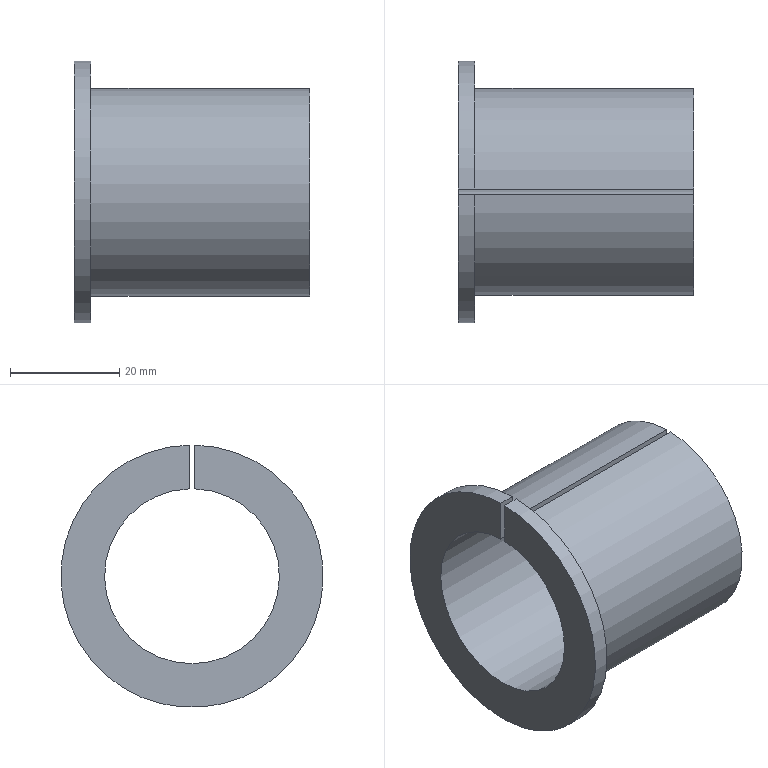Part | STEP file | HXGR200008-05-22-05 | 1 solid | 8 faces | box 43 x 48 x 47.995 mm | volume 16067 mm3 | plane 5 | cylinder 3 | commonest cylinder face diameters 32 x1 38 x1 48 x1
STEP:
#1=CARTESIAN_POINT('',(0.,0.5,23.995));
#2=VERTEX_POINT('',#1);
#3=CARTESIAN_POINT('',(0.,-0.5,23.995));
#4=VERTEX_POINT('',#3);
#5=CARTESIAN_POINT('',(0.,0.,0.));
#6=DIRECTION('',(-1.,0.,0.));
#7=DIRECTION('',(0.,0.,1.));
#8=AXIS2_PLACEMENT_3D('',#5,#6,#7);
#9=CIRCLE('',#8,24.);
#10=EDGE_CURVE('',#2,#4,#9,.T.);
#11=ORIENTED_EDGE('',*,*,#10,.F.);
#12=CARTESIAN_POINT('',(3.,0.5,23.995));
#13=VERTEX_POINT('',#12);
#14=CARTESIAN_POINT('',(0.,0.5,23.995));
#15=DIRECTION('',(-1.,0.,0.));
#16=VECTOR('',#15,1000.);
#17=LINE('',#14,#16);
#18=EDGE_CURVE('',#13,#2,#17,.T.);
#19=ORIENTED_EDGE('',*,*,#18,.F.);
#20=CARTESIAN_POINT('',(3.,-0.5,23.995));
#21=VERTEX_POINT('',#20);
#22=CARTESIAN_POINT('',(3.,0.,0.));
#23=DIRECTION('',(-1.,0.,0.));
#24=DIRECTION('',(0.,0.,1.));
#25=AXIS2_PLACEMENT_3D('',#22,#23,#24);
#26=CIRCLE('',#25,24.);
#27=EDGE_CURVE('',#13,#21,#26,.T.);
#28=ORIENTED_EDGE('',*,*,#27,.T.);
#29=CARTESIAN_POINT('',(0.,-0.5,23.995));
#30=DIRECTION('',(1.,0.,0.));
#31=VECTOR('',#30,1000.);
#32=LINE('',#29,#31);
#33=EDGE_CURVE('',#4,#21,#32,.T.);
#34=ORIENTED_EDGE('',*,*,#33,.F.);
#35=EDGE_LOOP('',(#11,#19,#28,#34));
#36=FACE_OUTER_BOUND('',#35,.T.);
#37=CARTESIAN_POINT('',(0.,0.,0.));
#38=DIRECTION('',(-1.,0.,0.));
#39=DIRECTION('',(0.,0.,1.));
#40=AXIS2_PLACEMENT_3D('',#37,#38,#39);
#41=CYLINDRICAL_SURFACE('',#40,24.);
#42=ADVANCED_FACE('',(#36),#41,.T.);
#43=CARTESIAN_POINT('',(0.,0.5,15.992));
#44=VERTEX_POINT('',#43);
#45=CARTESIAN_POINT('',(0.,-0.5,15.992));
#46=VERTEX_POINT('',#45);
#47=CARTESIAN_POINT('',(0.,0.,0.));
#48=DIRECTION('',(-1.,0.,0.));
#49=DIRECTION('',(0.,0.,1.));
#50=AXIS2_PLACEMENT_3D('',#47,#48,#49);
#51=CIRCLE('',#50,16.);
#52=EDGE_CURVE('',#44,#46,#51,.T.);
#53=ORIENTED_EDGE('',*,*,#52,.F.);
#54=CARTESIAN_POINT('',(0.,0.5,48.));
#55=DIRECTION('',(0.,0.,-1.));
#56=VECTOR('',#55,1000.);
#57=LINE('',#54,#56);
#58=EDGE_CURVE('',#2,#44,#57,.T.);
#59=ORIENTED_EDGE('',*,*,#58,.F.);
#60=ORIENTED_EDGE('',*,*,#10,.T.);
#61=CARTESIAN_POINT('',(0.,-0.5,48.));
#62=DIRECTION('',(0.,0.,1.));
#63=VECTOR('',#62,1000.);
#64=LINE('',#61,#63);
#65=EDGE_CURVE('',#46,#4,#64,.T.);
#66=ORIENTED_EDGE('',*,*,#65,.F.);
#67=EDGE_LOOP('',(#53,#59,#60,#66));
#68=FACE_OUTER_BOUND('',#67,.T.);
#69=CARTESIAN_POINT('',(0.,24.,0.));
#70=DIRECTION('',(1.,0.,0.));
#71=DIRECTION('',(0.,0.,-1.));
#72=AXIS2_PLACEMENT_3D('',#69,#70,#71);
#73=PLANE('',#72);
#74=ADVANCED_FACE('',(#68),#73,.F.);
#75=CARTESIAN_POINT('',(43.,0.5,15.992));
#76=VERTEX_POINT('',#75);
#77=CARTESIAN_POINT('',(43.,-0.5,15.992));
#78=VERTEX_POINT('',#77);
#79=CARTESIAN_POINT('',(43.,0.,0.));
#80=DIRECTION('',(-1.,0.,0.));
#81=DIRECTION('',(0.,0.,1.));
#82=AXIS2_PLACEMENT_3D('',#79,#80,#81);
#83=CIRCLE('',#82,16.);
#84=EDGE_CURVE('',#76,#78,#83,.T.);
#85=ORIENTED_EDGE('',*,*,#84,.F.);
#86=CARTESIAN_POINT('',(0.,0.5,15.992));
#87=DIRECTION('',(1.,0.,0.));
#88=VECTOR('',#87,1000.);
#89=LINE('',#86,#88);
#90=EDGE_CURVE('',#44,#76,#89,.T.);
#91=ORIENTED_EDGE('',*,*,#90,.F.);
#92=ORIENTED_EDGE('',*,*,#52,.T.);
#93=CARTESIAN_POINT('',(0.,-0.5,15.992));
#94=DIRECTION('',(-1.,0.,0.));
#95=VECTOR('',#94,1000.);
#96=LINE('',#93,#95);
#97=EDGE_CURVE('',#78,#46,#96,.T.);
#98=ORIENTED_EDGE('',*,*,#97,.F.);
#99=EDGE_LOOP('',(#85,#91,#92,#98));
#100=FACE_OUTER_BOUND('',#99,.T.);
#101=CARTESIAN_POINT('',(0.,0.,0.));
#102=DIRECTION('',(-1.,0.,0.));
#103=DIRECTION('',(0.,0.,1.));
#104=AXIS2_PLACEMENT_3D('',#101,#102,#103);
#105=CYLINDRICAL_SURFACE('',#104,16.);
#106=ADVANCED_FACE('',(#100),#105,.F.);
#107=CARTESIAN_POINT('',(43.,0.5,18.993));
#108=VERTEX_POINT('',#107);
#109=CARTESIAN_POINT('',(43.,-0.5,18.993));
#110=VERTEX_POINT('',#109);
#111=CARTESIAN_POINT('',(43.,0.,0.));
#112=DIRECTION('',(-1.,0.,0.));
#113=DIRECTION('',(0.,0.,1.));
#114=AXIS2_PLACEMENT_3D('',#111,#112,#113);
#115=CIRCLE('',#114,19.);
#116=EDGE_CURVE('',#108,#110,#115,.T.);
#117=ORIENTED_EDGE('',*,*,#116,.F.);
#118=CARTESIAN_POINT('',(43.,0.5,48.));
#119=DIRECTION('',(0.,0.,1.));
#120=VECTOR('',#119,1000.);
#121=LINE('',#118,#120);
#122=EDGE_CURVE('',#76,#108,#121,.T.);
#123=ORIENTED_EDGE('',*,*,#122,.F.);
#124=ORIENTED_EDGE('',*,*,#84,.T.);
#125=CARTESIAN_POINT('',(43.,-0.5,48.));
#126=DIRECTION('',(0.,0.,-1.));
#127=VECTOR('',#126,1000.);
#128=LINE('',#125,#127);
#129=EDGE_CURVE('',#110,#78,#128,.T.);
#130=ORIENTED_EDGE('',*,*,#129,.F.);
#131=EDGE_LOOP('',(#117,#123,#124,#130));
#132=FACE_OUTER_BOUND('',#131,.T.);
#133=CARTESIAN_POINT('',(43.,16.,0.));
#134=DIRECTION('',(-1.,0.,0.));
#135=DIRECTION('',(0.,0.,1.));
#136=AXIS2_PLACEMENT_3D('',#133,#134,#135);
#137=PLANE('',#136);
#138=ADVANCED_FACE('',(#132),#137,.F.);
#139=CARTESIAN_POINT('',(3.,0.5,18.993));
#140=VERTEX_POINT('',#139);
#141=CARTESIAN_POINT('',(3.,-0.5,18.993));
#142=VERTEX_POINT('',#141);
#143=CARTESIAN_POINT('',(3.,0.,0.));
#144=DIRECTION('',(-1.,0.,0.));
#145=DIRECTION('',(0.,0.,1.));
#146=AXIS2_PLACEMENT_3D('',#143,#144,#145);
#147=CIRCLE('',#146,19.);
#148=EDGE_CURVE('',#140,#142,#147,.T.);
#149=ORIENTED_EDGE('',*,*,#148,.F.);
#150=CARTESIAN_POINT('',(0.,0.5,18.993));
#151=DIRECTION('',(-1.,0.,0.));
#152=VECTOR('',#151,1000.);
#153=LINE('',#150,#152);
#154=EDGE_CURVE('',#108,#140,#153,.T.);
#155=ORIENTED_EDGE('',*,*,#154,.F.);
#156=ORIENTED_EDGE('',*,*,#116,.T.);
#157=CARTESIAN_POINT('',(0.,-0.5,18.993));
#158=DIRECTION('',(1.,0.,0.));
#159=VECTOR('',#158,1000.);
#160=LINE('',#157,#159);
#161=EDGE_CURVE('',#142,#110,#160,.T.);
#162=ORIENTED_EDGE('',*,*,#161,.F.);
#163=EDGE_LOOP('',(#149,#155,#156,#162));
#164=FACE_OUTER_BOUND('',#163,.T.);
#165=CARTESIAN_POINT('',(0.,0.,0.));
#166=DIRECTION('',(-1.,0.,0.));
#167=DIRECTION('',(0.,0.,1.));
#168=AXIS2_PLACEMENT_3D('',#165,#166,#167);
#169=CYLINDRICAL_SURFACE('',#168,19.);
#170=ADVANCED_FACE('',(#164),#169,.T.);
#171=ORIENTED_EDGE('',*,*,#27,.F.);
#172=CARTESIAN_POINT('',(3.,0.5,48.));
#173=DIRECTION('',(0.,0.,1.));
#174=VECTOR('',#173,1000.);
#175=LINE('',#172,#174);
#176=EDGE_CURVE('',#140,#13,#175,.T.);
#177=ORIENTED_EDGE('',*,*,#176,.F.);
#178=ORIENTED_EDGE('',*,*,#148,.T.);
#179=CARTESIAN_POINT('',(3.,-0.5,48.));
#180=DIRECTION('',(0.,0.,-1.));
#181=VECTOR('',#180,1000.);
#182=LINE('',#179,#181);
#183=EDGE_CURVE('',#21,#142,#182,.T.);
#184=ORIENTED_EDGE('',*,*,#183,.F.);
#185=EDGE_LOOP('',(#171,#177,#178,#184));
#186=FACE_OUTER_BOUND('',#185,.T.);
#187=CARTESIAN_POINT('',(3.,19.,0.));
#188=DIRECTION('',(-1.,0.,0.));
#189=DIRECTION('',(0.,0.,1.));
#190=AXIS2_PLACEMENT_3D('',#187,#188,#189);
#191=PLANE('',#190);
#192=ADVANCED_FACE('',(#186),#191,.F.);
#193=ORIENTED_EDGE('',*,*,#33,.T.);
#194=ORIENTED_EDGE('',*,*,#183,.T.);
#195=ORIENTED_EDGE('',*,*,#161,.T.);
#196=ORIENTED_EDGE('',*,*,#129,.T.);
#197=ORIENTED_EDGE('',*,*,#97,.T.);
#198=ORIENTED_EDGE('',*,*,#65,.T.);
#199=EDGE_LOOP('',(#193,#194,#195,#196,#197,#198));
#200=FACE_OUTER_BOUND('',#199,.T.);
#201=CARTESIAN_POINT('',(43.001,-0.5,48.));
#202=DIRECTION('',(0.,-1.,0.));
#203=DIRECTION('',(0.,0.,-1.));
#204=AXIS2_PLACEMENT_3D('',#201,#202,#203);
#205=PLANE('',#204);
#206=ADVANCED_FACE('',(#200),#205,.F.);
#207=ORIENTED_EDGE('',*,*,#18,.T.);
#208=ORIENTED_EDGE('',*,*,#58,.T.);
#209=ORIENTED_EDGE('',*,*,#90,.T.);
#210=ORIENTED_EDGE('',*,*,#122,.T.);
#211=ORIENTED_EDGE('',*,*,#154,.T.);
#212=ORIENTED_EDGE('',*,*,#176,.T.);
#213=EDGE_LOOP('',(#207,#208,#209,#210,#211,#212));
#214=FACE_OUTER_BOUND('',#213,.T.);
#215=CARTESIAN_POINT('',(43.001,0.5,48.));
#216=DIRECTION('',(0.,1.,0.));
#217=DIRECTION('',(0.,0.,1.));
#218=AXIS2_PLACEMENT_3D('',#215,#216,#217);
#219=PLANE('',#218);
#220=ADVANCED_FACE('',(#214),#219,.F.);
#221=CLOSED_SHELL('',(#42,#74,#106,#138,#170,#192,#206,#220));
#222=MANIFOLD_SOLID_BREP('',#221);
#223=CARTESIAN_POINT('',(0.,0.,0.));
#224=DIRECTION('',(0.,0.,1.));
#225=DIRECTION('',(1.,0.,0.));
#226=AXIS2_PLACEMENT_3D('',#223,#224,#225);
#227=(LENGTH_UNIT()NAMED_UNIT(*)SI_UNIT(.MILLI.,.METRE.));
#228=UNCERTAINTY_MEASURE_WITH_UNIT(LENGTH_MEASURE(0.00001),#227,'','');
#229=(NAMED_UNIT(*)PLANE_ANGLE_UNIT()SI_UNIT($,.RADIAN.));
#230=(NAMED_UNIT(*)SI_UNIT($,.STERADIAN.)SOLID_ANGLE_UNIT());
#231=(GEOMETRIC_REPRESENTATION_CONTEXT(3)GLOBAL_UNCERTAINTY_ASSIGNED_CONTEXT((#228))GLOBAL_UNIT_ASSIGNED_CONTEXT((#227,#229,#230))REPRESENTATION_CONTEXT('',''));
#232=ADVANCED_BREP_SHAPE_REPRESENTATION('',(#222,#226),#231);